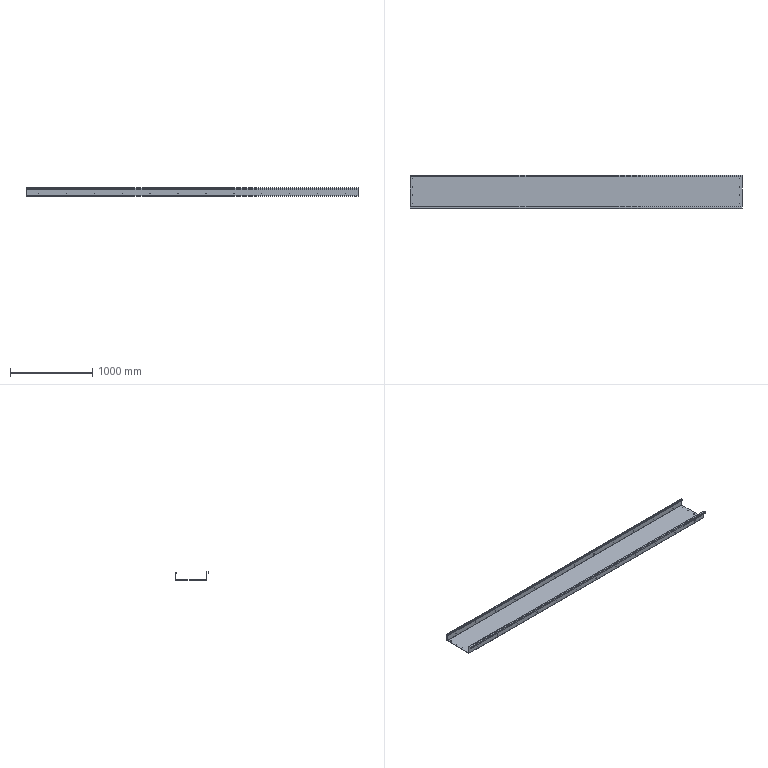Part | STEP file | TS-S44 | 1 solid | 118 faces | box 4045 x 403 x 100 mm | volume 5175456 mm3 | cylinder 76 | plane 42 | commonest cylinder face diameters 5.4 x48 5 x16 0.4 x6 4.4 x6